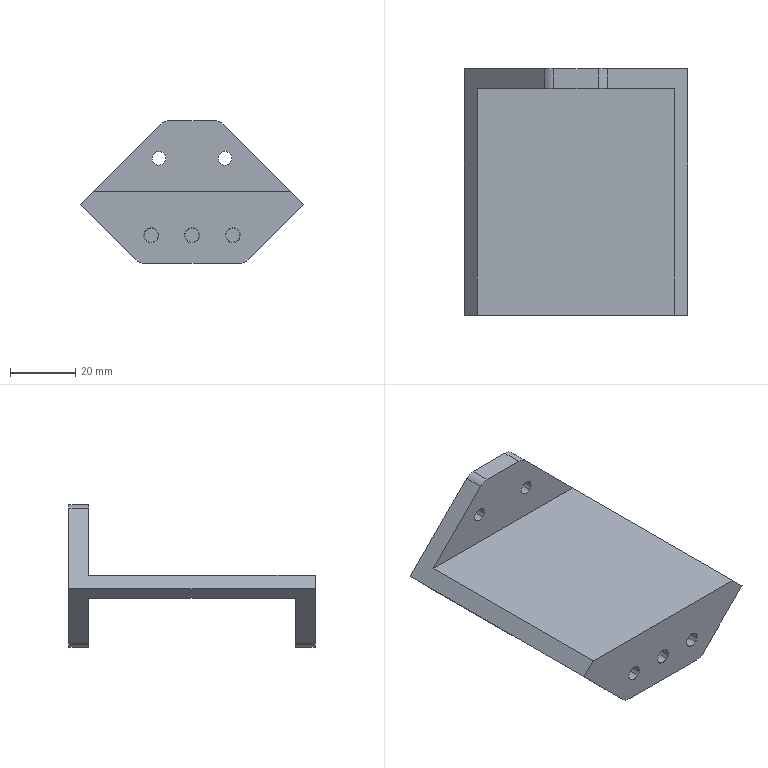NC program | NX | posted with a generic post | part box 68.307 x 75.3 x 43.668 mm
Lines 3784 to 3890 of 9000:
(ZLEVEL_PROFILE_COPY_1_COPY_COPY_1_COPY , TOOL : D10JING)
N7548 T14 M6
N7550 G54
N7552 G17 G0 G90 X39.271 Y-40.958 B0. C0. S9500 M3
N7554 G43 Z30. H14
N7556 Z-13.556
N7558 G94 G1 Z-14.556 F1000.
N7560 X38.515 Y-39.648
N7562 G3 X37.649 Y-39.148 R1.
N7564 G1 X-37.649 F1200.
N7566 G2 X-42.65 Y-34.147 R5.001
N7568 G1 Y34.147
N7570 G2 X-37.648 Y39.148 R5.002
N7572 G1 X37.649
N7574 G2 X42.65 Y34.147 R5.001
N7576 G1 Y-34.147
N7578 G2 X37.649 Y-39.148 R5.001
N7580 G3 X36.783 Y-39.648 R1.
N7582 G1 X35.917 Y-41.148
N7584 Z-13.556
N7586 G0 Z30.
N7588 X39.271 Y-40.958
N7590 Z-28.112
N7592 G1 Z-29.112 F1000.
N7594 X38.515 Y-39.648
N7596 G3 X37.649 Y-39.148 R1.
N7598 G1 X-37.649 F1200.
N7600 G2 X-42.65 Y-34.147 R5.001
N7602 G1 Y34.147
N7604 G2 X-37.648 Y39.148 R5.002
N7606 G1 X37.649
N7608 G2 X42.65 Y34.147 R5.001
N7610 G1 Y-34.147
N7612 G2 X37.649 Y-39.148 R5.001
N7614 G3 X36.783 Y-39.648 R1.
N7616 G1 X35.917 Y-41.148
N7618 Z-28.112
N7620 G0 Z30.
N7622 X39.271 Y-40.958
N7624 Z-42.668
N7626 G1 Z-43.668 F1000.
N7628 X38.515 Y-39.648
N7630 G3 X37.649 Y-39.148 R1.
N7632 G1 X-37.649 F1200.
N7634 G2 X-42.65 Y-34.147 R5.001
N7636 G1 Y34.147
N7638 G2 X-37.648 Y39.148 R5.002
N7640 G1 X37.649
N7642 G2 X42.65 Y34.147 R5.001
N7644 G1 Y-34.147
N7646 G2 X37.649 Y-39.148 R5.001
N7648 G3 X36.783 Y-39.648 R1.
N7650 G1 X35.917 Y-41.148
N7652 Z-42.668
N7654 G0 Z30.
(FLOOR_WALL_1 , TOOL : D10JING)
N7656 X-26.147 Y-39.153
N7658 Z-12.
N7660 G1 Z-15. F1250.
N7662 Y-36.153
N7664 Y36.153
N7666 X-21.393
N7668 Y-36.153
N7670 X-16.638
N7672 Y36.153
N7674 X-11.884
N7676 Y-36.153
N7678 X-7.13
N7680 Y36.153
N7682 X-2.376
N7684 Y-36.153
N7686 X2.379
N7688 Y36.153
N7690 X7.133
N7692 Y-36.153
N7694 X11.887
N7696 Y36.153
N7698 X16.641
N7700 Y-36.153
N7702 X21.396
N7704 Y36.153
N7706 X26.15
N7708 Y-36.153
N7710 Y-39.153
N7712 Z-12.
N7714 G0 Z30.
N7716 X26.65
N7718 Z-12.
N7720 G1 Z-15.
N7722 Y-36.153
N7724 Y36.153
N7726 Y39.153
N7728 Z-12.
N7730 G0 Z30.
N7732 X-26.65
N7734 Z-12.
N7736 G1 Z-15.
N7738 Y36.153
N7740 Y-36.153
N7742 Y-39.153
N7744 Z-12.
N7746 G0 Z30.
N7748 M5